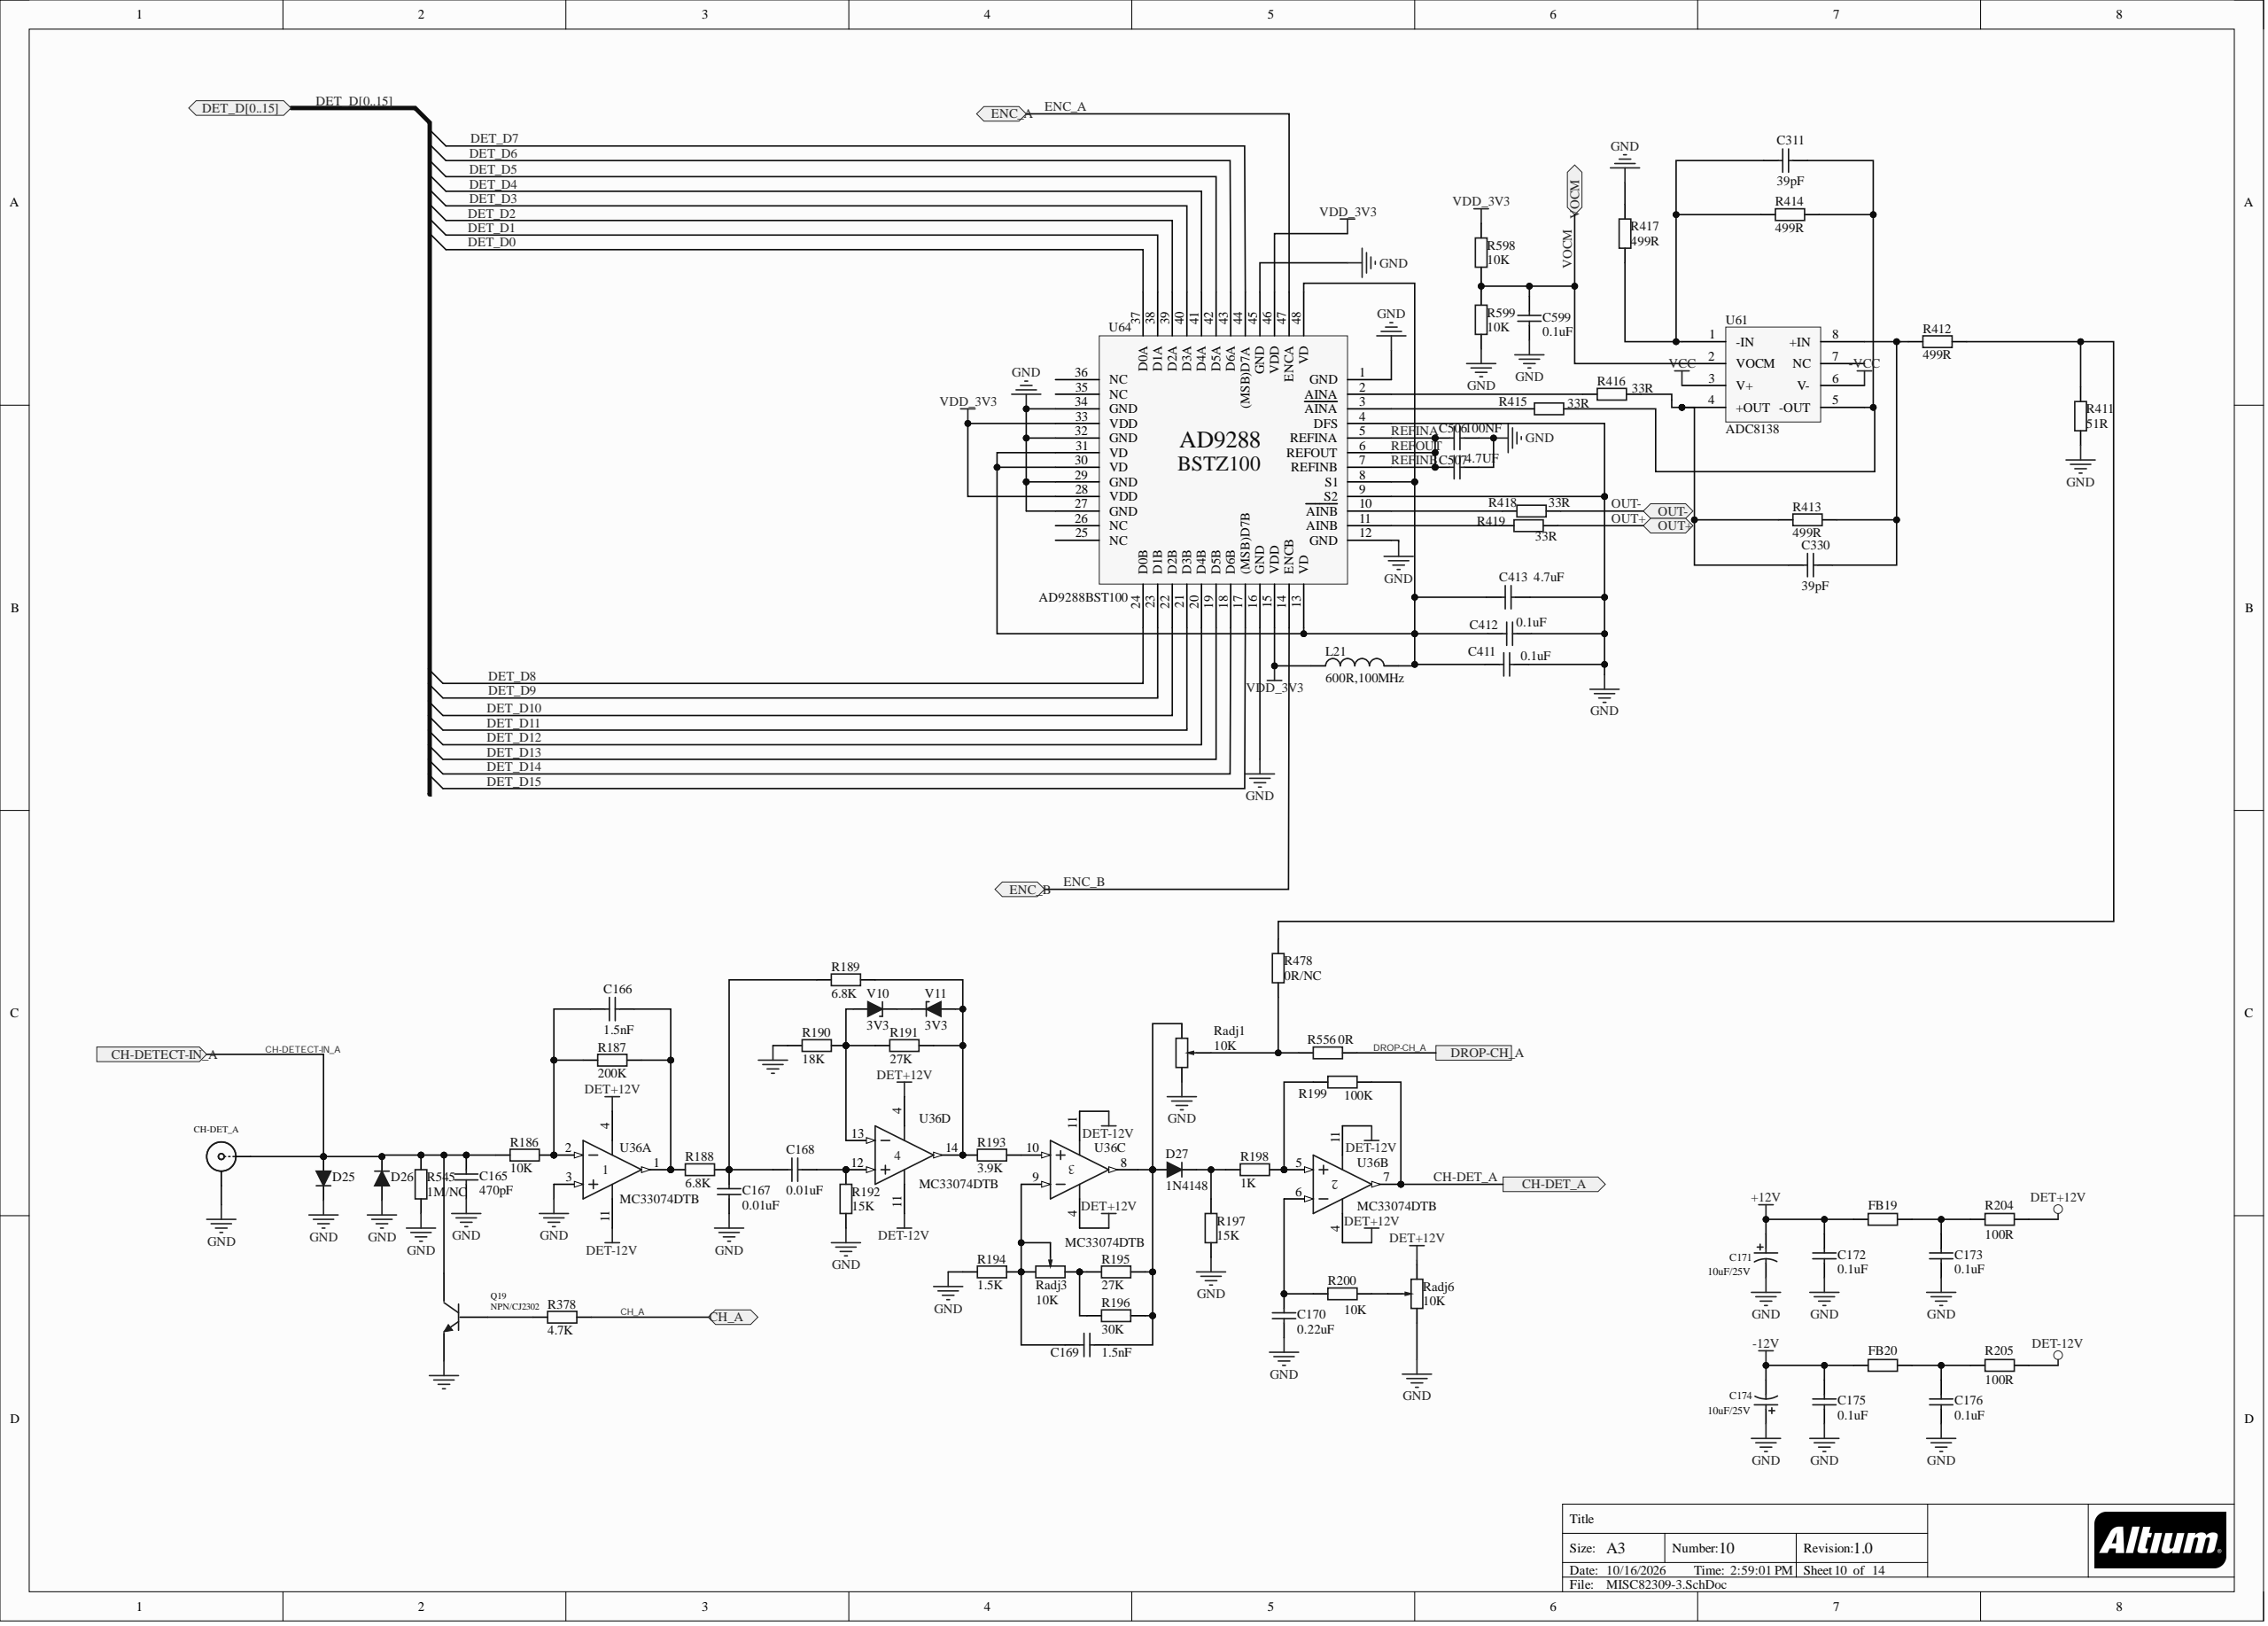Circuit board | Altium Designer | 747 parts | 576 nets | one sheet of the schematic
Parts on this sheet (reference | value | footprint):
C165 | 470pF | C0603
C166 | 1.5nF | C0603
C167 | 0.01uF | C0603
C168 | 0.01uF | C0603
C169 | 1.5nF | C0603
C170 | 0.22uF | C0603
C171 | 10uF/25V | E5X5.4
C172 | 0.1uF | C0805
C173 | 0.1uF | C0805
C174 | 10uF/25V | E5X5.4
C175 | 0.1uF | C0805
C176 | 0.1uF | C0805
C311 | 39pF | CAP_0603
C330 | 39pF | CAP_0603
C411 | 0.1uF | CAP_0603
C412 | 0.1uF | CAP_0603
C413 | 4.7uF | CAP_0603
C599 | 0.1uF | CAP_0603
CH-DET_A | SMB | SMB_V-RJ45
D25 | 1N4148WS | SOD323
D26 | 1N4148WS | SOD323
D27 | 1N4148 | SOD-323
FB19 | 60 | SMD0805-L
FB20 | 60 | SMD0805-L
L21 | 600R,100MHz | R0805
Q19 | NPN/CJ2302 | SOT-23-3
R186 | 10K | RES_0603
R187 | 200K | RES_0603
R188 | 6.8K | RES_0603
R189 | 6.8K | RES_0603
R190 | 18K | RES_0603
R191 | 27K | RES_0603
R192 | 15K | RES_0603
R193 | 3.9K | RES_0603
R194 | 1.5K | RES_0603
R195 | 27K | RES_0603
R196 | 30K | RES_0603
R197 | 15K | RES_0603
R198 | 1K | RES_0603
R199 | 100K | RES_0603
R200 | 10K | RES_0603
R204 | 100R | R0805
R205 | 100R | R0805
R378 | 4.7K | RES_0603
R411 | 51R | RES_0603
R412 | 499R | RES_0603
R413 | 499R | RES_0603
R414 | 499R | RES_0603
R415 | 33R | RES_0603
R416 | 33R | RES_0603
R417 | 499R | RES_0603
R418 | 33R | RES_0603
R419 | 33R | RES_0603
R478 | 0R/NC | RES_0603
R545 | 1M/NC | RES_0603
R556 | 0R | RES_0603
R598 | 10K | RES_0603
R599 | 10K | RES_0603
Radj1 | 10K | Radj
Radj3 | 10K | Radj
Radj6 | 10K | Radj
U61 | ADC8138 | SO8
U64 | AD9288BST100 | LQFP48A
V10 | 3V3 | SOD-123
V11 | 3V3 | SOD-123
Nets of these parts (net: part-pin ...):
VOCM: C599-1 R598-1 R599-2 U61-2
VDD_3V3: L21-2 R598-2 U64-15 U64-28 U64-33 U64-46
VCC: U61-3
REFINA: U64-5 U64-6 U64-7
OUT-: R418-2
OUT+: R419-1
NetV10_2: V10-2 V11-2
NetR478_1: R478-1 R556-2 Radj1-2
NetR419_2: R419-2 U64-11
NetR418_1: R418-1 U64-10
NetR416_1: R416-1 U64-2
NetR415_2: R415-2 U64-3
NetR411_1: R411-1 R412-2 R478-2
NetR200_2: R200-2 Radj6-2
NetR198_2: R198-2 R199-1
NetR195_1: R195-1 R196-1 Radj3-1
NetR193_1: R193-1
NetR190_2: R190-2 R191-1 V10-1
NetR189_2: R189-2 R191-2 R193-2 V11-1
NetQ19_1: Q19-1 R378-1
NetD27_2: D27-2 R197-2 R198-1
NetC411_2: C411-2 C412-2 C413-2 L21-1 U64-8 U64-13 U64-30 U64-31 U64-48
NetC330_2: C330-2 R412-1 R413-2 U61-8
NetC330_1: C330-1 R413-1 R416-2 U61-4
NetC311_2: C311-2 R414-2 R417-1 U61-1
NetC311_1: C311-1 R414-1 R415-1 U61-5
NetC176_2: C176-2 FB20-2 R205-1
NetC173_2: C173-2 FB19-2 R204-1
NetC170_1: C170-1 R200-1
NetC169_2: C169-2 R194-2 Radj3-2 Radj3-3
NetC169_1: C169-1 D27-1 R195-2 R196-2 Radj1-3
NetC168_1: C168-1 R192-2
NetC167_1: C167-1 C168-2 R188-2 R189-1
NetC166_2: C166-2 R186-2 R187-1
NetC166_1: C166-1 R187-2 R188-1
GND: C165-1 C167-2 C170-2 C171-2 C172-1 C173-1 C174-1 C175-1 C176-1 C411-1 C412-1 C413-1 C599-2 CH-DET_A-2 D25-2 D26-1 Q19-2 R190-1 R192-1 R194-1 R197-1 R411-2 R417-2 R545-1 R599-1 Radj1-1 Radj6-1 U64-1 U64-4 U64-9 U64-12 U64-16 U64-27 U64-29 U64-32 U64-34 U64-45
ENC_B: U64-14
ENC_A: U64-47
DROP-CH_A: R556-1
DET_D15: U64-17
DET_D14: U64-18
DET_D13: U64-19
DET_D12: U64-20
DET_D11: U64-21
DET_D10: U64-22
DET_D9: U64-23
DET_D8: U64-24
DET_D7: U64-44
DET_D6: U64-43
DET_D5: U64-42
DET_D4: U64-41
DET_D3: U64-40
DET_D2: U64-39
DET_D1: U64-38
DET_D0: U64-37
DET-12V: R205-2
DET+12V: R204-2 Radj6-3
CH_A: R378-2
CH-DETECT-IN_A: C165-2 CH-DET_A-1 D25-1 D26-2 Q19-3 R186-1 R545-2
CH-DET_A: R199-2
-VCC: U61-6
-12V: C174-2 C175-2 FB20-1
+12V: C171-1 C172-2 FB19-1